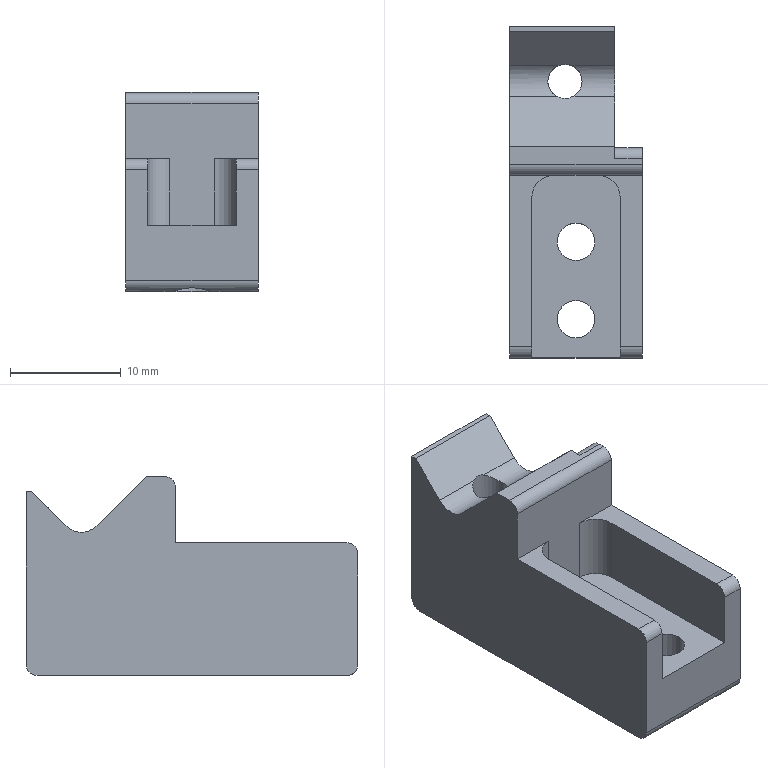Part | STEP file | 1 solid | 42 faces | box 12 x 30 x 18 mm | volume 3302 mm3 | cylinder 23 | plane 19 | commonest cylinder face diameters 2 x7 3.4 x4 4 x4 6.5 x4 2.5 x2 3.1 x2